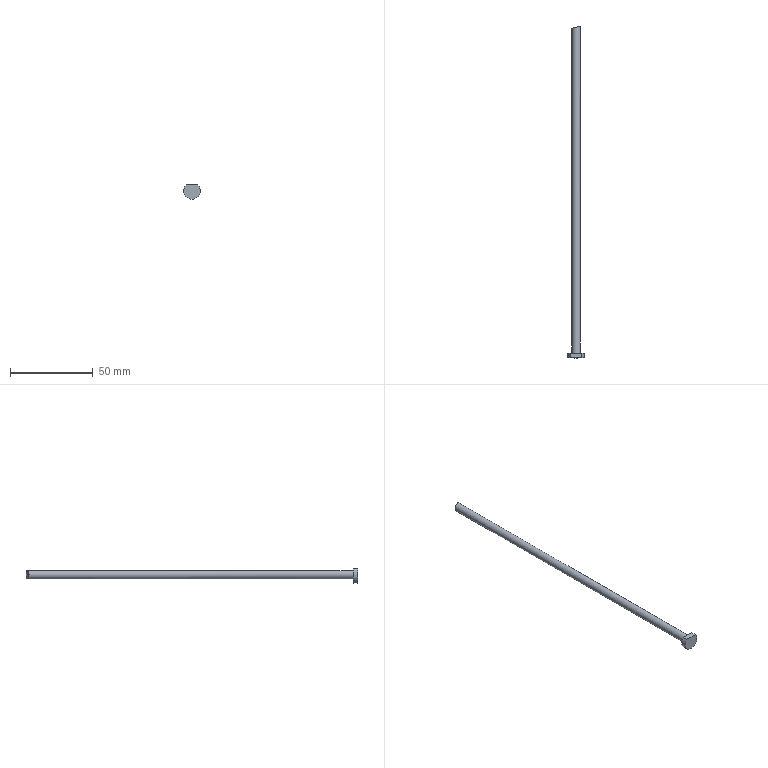Part | STEP file | EJECTION-PIN_id146_x_t | 1 solid | 8 faces | box 10 x 200.49 x 8.5 mm | volume 4074 mm3 | plane 3 | other 2 | cylinder 2 | spline 1 | commonest cylinder face diameters 5 x1 10 x1
STEP:
#1=CARTESIAN_POINT('',(22.131,-220.5,23.73));
#2=VERTEX_POINT('',#1);
#3=CARTESIAN_POINT('',(14.989,-220.5,23.73));
#4=VERTEX_POINT('',#3);
#5=CARTESIAN_POINT('',(18.56,-220.5,20.23));
#6=DIRECTION('',(0.,1.,0.));
#7=DIRECTION('',(0.,0.,1.));
#8=AXIS2_PLACEMENT_3D('',#5,#6,#7);
#9=CIRCLE('',#8,5.);
#10=EDGE_CURVE('',#2,#4,#9,.T.);
#11=ORIENTED_EDGE('',*,*,#10,.F.);
#12=CARTESIAN_POINT('',(14.989,-220.5,23.73));
#13=DIRECTION('',(1.,0.,0.));
#14=VECTOR('',#13,1.);
#15=LINE('',#12,#14);
#16=EDGE_CURVE('',#4,#2,#15,.T.);
#17=ORIENTED_EDGE('',*,*,#16,.F.);
#18=EDGE_LOOP('',(#11,#17));
#19=FACE_OUTER_BOUND('',#18,.T.);
#20=CARTESIAN_POINT('',(-30.,-220.5,27.));
#21=DIRECTION('',(0.,1.,0.));
#22=DIRECTION('',(0.,0.,1.));
#23=AXIS2_PLACEMENT_3D('',#20,#21,#22);
#24=PLANE('',#23);
#25=ADVANCED_FACE('',(#19),#24,.F.);
#26=CARTESIAN_POINT('',(16.073,-21.57,20.485));
#27=VERTEX_POINT('',#26);
#28=CARTESIAN_POINT('',(16.073,-21.57,19.976));
#29=VERTEX_POINT('',#28);
#30=CARTESIAN_POINT('',(16.073,-21.57,20.485));
#31=CARTESIAN_POINT('',(16.073,-21.595,20.485));
#32=CARTESIAN_POINT('',(16.073,-21.62,20.48));
#33=CARTESIAN_POINT('',(16.072,-21.644,20.473));
#34=CARTESIAN_POINT('',(16.071,-21.678,20.462));
#35=CARTESIAN_POINT('',(16.069,-21.711,20.446));
#36=CARTESIAN_POINT('',(16.068,-21.74,20.425));
#37=CARTESIAN_POINT('',(16.066,-21.761,20.408));
#38=CARTESIAN_POINT('',(16.065,-21.781,20.389));
#39=CARTESIAN_POINT('',(16.064,-21.797,20.366));
#40=CARTESIAN_POINT('',(16.062,-21.812,20.344));
#41=CARTESIAN_POINT('',(16.061,-21.824,20.318));
#42=CARTESIAN_POINT('',(16.061,-21.83,20.291));
#43=CARTESIAN_POINT('',(16.06,-21.835,20.271));
#44=CARTESIAN_POINT('',(16.06,-21.837,20.251));
#45=CARTESIAN_POINT('',(16.06,-21.837,20.23));
#46=CARTESIAN_POINT('',(16.06,-21.837,20.205));
#47=CARTESIAN_POINT('',(16.06,-21.834,20.18));
#48=CARTESIAN_POINT('',(16.061,-21.827,20.156));
#49=CARTESIAN_POINT('',(16.062,-21.818,20.129));
#50=CARTESIAN_POINT('',(16.063,-21.805,20.102));
#51=CARTESIAN_POINT('',(16.064,-21.787,20.08));
#52=CARTESIAN_POINT('',(16.066,-21.771,20.061));
#53=CARTESIAN_POINT('',(16.067,-21.752,20.044));
#54=CARTESIAN_POINT('',(16.068,-21.731,20.03));
#55=CARTESIAN_POINT('',(16.069,-21.707,20.013));
#56=CARTESIAN_POINT('',(16.071,-21.68,20.));
#57=CARTESIAN_POINT('',(16.072,-21.653,19.99));
#58=CARTESIAN_POINT('',(16.072,-21.626,19.981));
#59=CARTESIAN_POINT('',(16.073,-21.598,19.976));
#60=CARTESIAN_POINT('',(16.073,-21.57,19.976));
#61=B_SPLINE_CURVE_WITH_KNOTS('',3,(#30,#31,#32,#33,#34,#35,#36,#37,#38,#39,#40,#41,#42,#43,#44,#45,#46,#47,#48,#49,#50,#51,#52,#53,#54,#55,#56,#57,#58,#59,#60),.UNSPECIFIED.,.F.,.F.,(4,3,3,3,3,3,3,3,3,3,4),(0.,0.09209,0.2236,0.324,0.4253,0.5006,0.5924,0.6977,0.7892,0.8972,1.),.UNSPECIFIED.);
#62=EDGE_CURVE('',#27,#29,#61,.T.);
#63=ORIENTED_EDGE('',*,*,#62,.F.);
#64=CARTESIAN_POINT('',(21.047,-20.01,20.485));
#65=VERTEX_POINT('',#64);
#66=CARTESIAN_POINT('',(21.285,-19.924,20.485));
#67=CARTESIAN_POINT('',(20.558,-20.19,20.485));
#68=CARTESIAN_POINT('',(18.748,-20.805,20.485));
#69=CARTESIAN_POINT('',(16.921,-21.342,20.485));
#70=CARTESIAN_POINT('',(15.829,-21.636,20.485));
#71=B_SPLINE_CURVE_WITH_KNOTS('',3,(#66,#67,#68,#69,#70),.UNSPECIFIED.,.F.,.F.,(4,1,4),(0.,0.4054,1.),.UNSPECIFIED.);
#72=EDGE_CURVE('',#65,#27,#71,.T.);
#73=ORIENTED_EDGE('',*,*,#72,.F.);
#74=CARTESIAN_POINT('',(21.047,-20.01,19.976));
#75=VERTEX_POINT('',#74);
#76=CARTESIAN_POINT('',(21.047,-20.01,19.976));
#77=CARTESIAN_POINT('',(21.047,-20.035,19.976));
#78=CARTESIAN_POINT('',(21.047,-20.061,19.98));
#79=CARTESIAN_POINT('',(21.048,-20.085,19.987));
#80=CARTESIAN_POINT('',(21.049,-20.118,19.997));
#81=CARTESIAN_POINT('',(21.051,-20.15,20.013));
#82=CARTESIAN_POINT('',(21.052,-20.178,20.034));
#83=CARTESIAN_POINT('',(21.054,-20.2,20.05));
#84=CARTESIAN_POINT('',(21.055,-20.219,20.069));
#85=CARTESIAN_POINT('',(21.056,-20.235,20.091));
#86=CARTESIAN_POINT('',(21.057,-20.25,20.113));
#87=CARTESIAN_POINT('',(21.058,-20.262,20.139));
#88=CARTESIAN_POINT('',(21.059,-20.268,20.165));
#89=CARTESIAN_POINT('',(21.06,-20.274,20.186));
#90=CARTESIAN_POINT('',(21.06,-20.276,20.208));
#91=CARTESIAN_POINT('',(21.06,-20.276,20.23));
#92=CARTESIAN_POINT('',(21.06,-20.276,20.255));
#93=CARTESIAN_POINT('',(21.06,-20.273,20.28));
#94=CARTESIAN_POINT('',(21.059,-20.266,20.304));
#95=CARTESIAN_POINT('',(21.058,-20.259,20.328));
#96=CARTESIAN_POINT('',(21.057,-20.248,20.351));
#97=CARTESIAN_POINT('',(21.056,-20.234,20.371));
#98=CARTESIAN_POINT('',(21.055,-20.219,20.392));
#99=CARTESIAN_POINT('',(21.054,-20.201,20.409));
#100=CARTESIAN_POINT('',(21.052,-20.181,20.424));
#101=CARTESIAN_POINT('',(21.051,-20.153,20.445));
#102=CARTESIAN_POINT('',(21.049,-20.121,20.462));
#103=CARTESIAN_POINT('',(21.048,-20.088,20.472));
#104=CARTESIAN_POINT('',(21.047,-20.063,20.48));
#105=CARTESIAN_POINT('',(21.047,-20.037,20.485));
#106=CARTESIAN_POINT('',(21.047,-20.01,20.485));
#107=B_SPLINE_CURVE_WITH_KNOTS('',3,(#76,#77,#78,#79,#80,#81,#82,#83,#84,#85,#86,#87,#88,#89,#90,#91,#92,#93,#94,#95,#96,#97,#98,#99,#100,#101,#102,#103,#104,#105,#106),.UNSPECIFIED.,.F.,.F.,(4,3,3,3,3,3,3,3,3,3,4),(0.,0.09206,0.2207,0.3199,0.4198,0.4998,0.5915,0.6832,0.7746,0.9031,1.),.UNSPECIFIED.);
#108=EDGE_CURVE('',#75,#65,#107,.T.);
#109=ORIENTED_EDGE('',*,*,#108,.F.);
#110=CARTESIAN_POINT('',(15.829,-21.636,19.976));
#111=CARTESIAN_POINT('',(16.921,-21.342,19.976));
#112=CARTESIAN_POINT('',(18.748,-20.805,19.976));
#113=CARTESIAN_POINT('',(20.558,-20.19,19.976));
#114=CARTESIAN_POINT('',(21.285,-19.924,19.976));
#115=B_SPLINE_CURVE_WITH_KNOTS('',3,(#110,#111,#112,#113,#114),.UNSPECIFIED.,.F.,.F.,(4,1,4),(0.,0.5946,1.),.UNSPECIFIED.);
#116=EDGE_CURVE('',#29,#75,#115,.T.);
#117=ORIENTED_EDGE('',*,*,#116,.F.);
#118=EDGE_LOOP('',(#63,#73,#109,#117));
#119=FACE_OUTER_BOUND('',#118,.T.);
#120=CARTESIAN_POINT('',(15.461,-21.559,20.297));
#121=CARTESIAN_POINT('',(16.66,-21.241,20.297));
#122=CARTESIAN_POINT('',(18.673,-20.655,20.297));
#123=CARTESIAN_POINT('',(20.663,-19.975,20.297));
#124=CARTESIAN_POINT('',(21.465,-19.676,20.297));
#125=CARTESIAN_POINT('',(15.469,-21.588,20.557));
#126=CARTESIAN_POINT('',(16.668,-21.271,20.557));
#127=CARTESIAN_POINT('',(18.682,-20.684,20.557));
#128=CARTESIAN_POINT('',(20.673,-20.004,20.557));
#129=CARTESIAN_POINT('',(21.476,-19.705,20.557));
#130=CARTESIAN_POINT('',(15.555,-21.916,20.478));
#131=CARTESIAN_POINT('',(16.76,-21.597,20.478));
#132=CARTESIAN_POINT('',(18.783,-21.008,20.478));
#133=CARTESIAN_POINT('',(20.786,-20.324,20.478));
#134=CARTESIAN_POINT('',(21.594,-20.023,20.478));
#135=CARTESIAN_POINT('',(15.574,-21.986,20.23));
#136=CARTESIAN_POINT('',(16.779,-21.667,20.23));
#137=CARTESIAN_POINT('',(18.804,-21.077,20.23));
#138=CARTESIAN_POINT('',(20.81,-20.392,20.23));
#139=CARTESIAN_POINT('',(21.619,-20.09,20.23));
#140=CARTESIAN_POINT('',(15.556,-21.918,19.987));
#141=CARTESIAN_POINT('',(16.76,-21.599,19.987));
#142=CARTESIAN_POINT('',(18.783,-21.009,19.987));
#143=CARTESIAN_POINT('',(20.786,-20.325,19.987));
#144=CARTESIAN_POINT('',(21.595,-20.024,19.987));
#145=CARTESIAN_POINT('',(15.473,-21.604,19.908));
#146=CARTESIAN_POINT('',(16.673,-21.286,19.908));
#147=CARTESIAN_POINT('',(18.687,-20.699,19.908));
#148=CARTESIAN_POINT('',(20.678,-20.019,19.908));
#149=CARTESIAN_POINT('',(21.481,-19.72,19.908));
#150=CARTESIAN_POINT('',(15.462,-21.562,20.137));
#151=CARTESIAN_POINT('',(16.661,-21.245,20.137));
#152=CARTESIAN_POINT('',(18.674,-20.658,20.137));
#153=CARTESIAN_POINT('',(20.664,-19.978,20.137));
#154=CARTESIAN_POINT('',(21.466,-19.68,20.137));
#155=B_SPLINE_SURFACE_WITH_KNOTS('',3,3,((#120,#121,#122,#123,#124),(#125,#126,#127,#128,#129),(#130,#131,#132,#133,#134),(#135,#136,#137,#138,#139),(#140,#141,#142,#143,#144),(#145,#146,#147,#148,#149),(#150,#151,#152,#153,#154)),.UNSPECIFIED.,.F.,.F.,.F.,(4,1,1,1,4),(4,1,4),(0.,0.3451,0.5061,0.667,1.),(0.,0.5922,1.),.UNSPECIFIED.);
#156=ADVANCED_FACE('',(#119),#155,.F.);
#157=ORIENTED_EDGE('',*,*,#72,.T.);
#158=CARTESIAN_POINT('',(21.047,-20.01,20.485));
#159=CARTESIAN_POINT('',(21.019,-20.02,20.754));
#160=CARTESIAN_POINT('',(20.946,-20.047,21.022));
#161=CARTESIAN_POINT('',(20.835,-20.086,21.266));
#162=CARTESIAN_POINT('',(20.724,-20.126,21.51));
#163=CARTESIAN_POINT('',(20.572,-20.179,21.737));
#164=CARTESIAN_POINT('',(20.393,-20.241,21.93));
#165=CARTESIAN_POINT('',(20.208,-20.305,22.13));
#166=CARTESIAN_POINT('',(19.988,-20.38,22.299));
#167=CARTESIAN_POINT('',(19.752,-20.459,22.428));
#168=CARTESIAN_POINT('',(19.503,-20.541,22.563));
#169=CARTESIAN_POINT('',(19.229,-20.631,22.655));
#170=CARTESIAN_POINT('',(18.951,-20.719,22.699));
#171=CARTESIAN_POINT('',(18.663,-20.811,22.745));
#172=CARTESIAN_POINT('',(18.363,-20.904,22.739));
#173=CARTESIAN_POINT('',(18.076,-20.992,22.683));
#174=CARTESIAN_POINT('',(17.788,-21.08,22.626));
#175=CARTESIAN_POINT('',(17.505,-21.164,22.516));
#176=CARTESIAN_POINT('',(17.251,-21.238,22.36));
#177=CARTESIAN_POINT('',(17.004,-21.31,22.208));
#178=CARTESIAN_POINT('',(16.779,-21.374,22.009));
#179=CARTESIAN_POINT('',(16.597,-21.425,21.778));
#180=CARTESIAN_POINT('',(16.422,-21.474,21.556));
#181=CARTESIAN_POINT('',(16.282,-21.513,21.298));
#182=CARTESIAN_POINT('',(16.191,-21.538,21.027));
#183=CARTESIAN_POINT('',(16.132,-21.554,20.852));
#184=CARTESIAN_POINT('',(16.092,-21.565,20.669));
#185=CARTESIAN_POINT('',(16.073,-21.57,20.485));
#186=B_SPLINE_CURVE_WITH_KNOTS('',3,(#158,#159,#160,#161,#162,#163,#164,#165,#166,#167,#168,#169,#170,#171,#172,#173,#174,#175,#176,#177,#178,#179,#180,#181,#182,#183,#184,#185),.UNSPECIFIED.,.F.,.F.,(4,3,3,3,3,3,3,3,3,4),(0.,0.1085,0.2168,0.3287,0.4468,0.569,0.6918,0.8115,0.9264,1.),.UNSPECIFIED.);
#187=EDGE_CURVE('',#65,#27,#186,.T.);
#188=ORIENTED_EDGE('',*,*,#187,.F.);
#189=EDGE_LOOP('',(#157,#188));
#190=FACE_OUTER_BOUND('',#189,.T.);
#191=CARTESIAN_POINT('',(15.829,-21.636,25.066));
#192=CARTESIAN_POINT('',(16.921,-21.342,25.066));
#193=CARTESIAN_POINT('',(18.748,-20.805,25.066));
#194=CARTESIAN_POINT('',(20.558,-20.19,25.066));
#195=CARTESIAN_POINT('',(21.285,-19.924,25.066));
#196=(BOUNDED_CURVE()B_SPLINE_CURVE(3,(#191,#192,#193,#194,#195),.UNSPECIFIED.,.F.,.F.)B_SPLINE_CURVE_WITH_KNOTS((4,1,4),(0.,0.5946,1.),.UNSPECIFIED.)CURVE()GEOMETRIC_REPRESENTATION_ITEM()RATIONAL_B_SPLINE_CURVE((1.,1.,1.,1.,1.))REPRESENTATION_ITEM(''));
#197=DIRECTION('',(0.,0.,-1.));
#198=VECTOR('',#197,1.);
#199=SURFACE_OF_LINEAR_EXTRUSION('',#196,#198);
#200=ADVANCED_FACE('',(#190),#199,.T.);
#201=CARTESIAN_POINT('',(14.989,-217.5,23.73));
#202=VERTEX_POINT('',#201);
#203=CARTESIAN_POINT('',(14.989,-220.5,23.73));
#204=DIRECTION('',(0.,1.,0.));
#205=VECTOR('',#204,1.);
#206=LINE('',#203,#205);
#207=EDGE_CURVE('',#4,#202,#206,.T.);
#208=ORIENTED_EDGE('',*,*,#207,.F.);
#209=ORIENTED_EDGE('',*,*,#16,.T.);
#210=CARTESIAN_POINT('',(22.131,-217.5,23.73));
#211=VERTEX_POINT('',#210);
#212=CARTESIAN_POINT('',(22.131,-220.5,23.73));
#213=DIRECTION('',(0.,-1.,0.));
#214=VECTOR('',#213,1.);
#215=LINE('',#212,#214);
#216=EDGE_CURVE('',#211,#2,#215,.T.);
#217=ORIENTED_EDGE('',*,*,#216,.F.);
#218=CARTESIAN_POINT('',(130.,-217.5,23.73));
#219=DIRECTION('',(1.,0.,0.));
#220=VECTOR('',#219,1.);
#221=LINE('',#218,#220);
#222=EDGE_CURVE('',#202,#211,#221,.T.);
#223=ORIENTED_EDGE('',*,*,#222,.F.);
#224=EDGE_LOOP('',(#208,#209,#217,#223));
#225=FACE_OUTER_BOUND('',#224,.T.);
#226=CARTESIAN_POINT('',(14.989,-220.5,23.73));
#227=DIRECTION('',(0.,0.,1.));
#228=DIRECTION('',(1.,0.,0.));
#229=AXIS2_PLACEMENT_3D('',#226,#227,#228);
#230=PLANE('',#229);
#231=ADVANCED_FACE('',(#225),#230,.T.);
#232=ORIENTED_EDGE('',*,*,#216,.T.);
#233=ORIENTED_EDGE('',*,*,#10,.T.);
#234=ORIENTED_EDGE('',*,*,#207,.T.);
#235=CARTESIAN_POINT('',(18.56,-217.5,20.23));
#236=DIRECTION('',(0.,1.,0.));
#237=DIRECTION('',(0.,0.,1.));
#238=AXIS2_PLACEMENT_3D('',#235,#236,#237);
#239=CIRCLE('',#238,5.);
#240=EDGE_CURVE('',#211,#202,#239,.T.);
#241=ORIENTED_EDGE('',*,*,#240,.F.);
#242=EDGE_LOOP('',(#232,#233,#234,#241));
#243=FACE_OUTER_BOUND('',#242,.T.);
#244=CARTESIAN_POINT('',(18.56,-220.5,20.23));
#245=DIRECTION('',(0.,1.,0.));
#246=DIRECTION('',(0.,0.,1.));
#247=AXIS2_PLACEMENT_3D('',#244,#245,#246);
#248=CYLINDRICAL_SURFACE('',#247,5.);
#249=ADVANCED_FACE('',(#243),#248,.T.);
#250=ORIENTED_EDGE('',*,*,#116,.T.);
#251=CARTESIAN_POINT('',(16.073,-21.57,19.976));
#252=CARTESIAN_POINT('',(16.101,-21.562,19.704));
#253=CARTESIAN_POINT('',(16.175,-21.542,19.433));
#254=CARTESIAN_POINT('',(16.289,-21.511,19.185));
#255=CARTESIAN_POINT('',(16.402,-21.479,18.939));
#256=CARTESIAN_POINT('',(16.558,-21.436,18.709));
#257=CARTESIAN_POINT('',(16.742,-21.384,18.513));
#258=CARTESIAN_POINT('',(16.93,-21.331,18.315));
#259=CARTESIAN_POINT('',(17.152,-21.267,18.146));
#260=CARTESIAN_POINT('',(17.391,-21.197,18.02));
#261=CARTESIAN_POINT('',(17.638,-21.124,17.89));
#262=CARTESIAN_POINT('',(17.909,-21.043,17.801));
#263=CARTESIAN_POINT('',(18.182,-20.96,17.759));
#264=CARTESIAN_POINT('',(18.465,-20.873,17.715));
#265=CARTESIAN_POINT('',(18.759,-20.781,17.722));
#266=CARTESIAN_POINT('',(19.04,-20.691,17.776));
#267=CARTESIAN_POINT('',(19.327,-20.599,17.833));
#268=CARTESIAN_POINT('',(19.608,-20.507,17.941));
#269=CARTESIAN_POINT('',(19.86,-20.422,18.095));
#270=CARTESIAN_POINT('',(20.111,-20.339,18.247));
#271=CARTESIAN_POINT('',(20.339,-20.26,18.448));
#272=CARTESIAN_POINT('',(20.523,-20.196,18.682));
#273=CARTESIAN_POINT('',(20.701,-20.134,18.907));
#274=CARTESIAN_POINT('',(20.843,-20.084,19.17));
#275=CARTESIAN_POINT('',(20.934,-20.051,19.446));
#276=CARTESIAN_POINT('',(20.99,-20.031,19.617));
#277=CARTESIAN_POINT('',(21.029,-20.017,19.796));
#278=CARTESIAN_POINT('',(21.047,-20.01,19.976));
#279=B_SPLINE_CURVE_WITH_KNOTS('',3,(#251,#252,#253,#254,#255,#256,#257,#258,#259,#260,#261,#262,#263,#264,#265,#266,#267,#268,#269,#270,#271,#272,#273,#274,#275,#276,#277,#278),.UNSPECIFIED.,.F.,.F.,(4,3,3,3,3,3,3,3,3,4),(0.,0.1095,0.2189,0.3303,0.4458,0.5657,0.6886,0.8107,0.9282,1.),.UNSPECIFIED.);
#280=EDGE_CURVE('',#29,#75,#279,.T.);
#281=ORIENTED_EDGE('',*,*,#280,.F.);
#282=EDGE_LOOP('',(#250,#281));
#283=FACE_OUTER_BOUND('',#282,.T.);
#284=CARTESIAN_POINT('',(15.829,-21.636,19.976));
#285=CARTESIAN_POINT('',(16.921,-21.342,19.976));
#286=CARTESIAN_POINT('',(18.748,-20.805,19.976));
#287=CARTESIAN_POINT('',(20.558,-20.19,19.976));
#288=CARTESIAN_POINT('',(21.285,-19.924,19.976));
#289=(BOUNDED_CURVE()B_SPLINE_CURVE(3,(#284,#285,#286,#287,#288),.UNSPECIFIED.,.F.,.F.)B_SPLINE_CURVE_WITH_KNOTS((4,1,4),(0.,0.5946,1.),.UNSPECIFIED.)CURVE()GEOMETRIC_REPRESENTATION_ITEM()RATIONAL_B_SPLINE_CURVE((1.,1.,1.,1.,1.))REPRESENTATION_ITEM(''));
#290=DIRECTION('',(0.,0.,-1.));
#291=VECTOR('',#290,1.);
#292=SURFACE_OF_LINEAR_EXTRUSION('',#289,#291);
#293=ADVANCED_FACE('',(#283),#292,.T.);
#294=CARTESIAN_POINT('',(18.56,-217.5,22.73));
#295=VERTEX_POINT('',#294);
#296=CARTESIAN_POINT('',(18.56,-217.5,20.23));
#297=DIRECTION('',(0.,1.,0.));
#298=DIRECTION('',(0.,0.,1.));
#299=AXIS2_PLACEMENT_3D('',#296,#297,#298);
#300=CIRCLE('',#299,2.5);
#301=EDGE_CURVE('',#295,#295,#300,.T.);
#302=ORIENTED_EDGE('',*,*,#301,.F.);
#303=EDGE_LOOP('',(#302));
#304=FACE_BOUND('',#303,.T.);
#305=ORIENTED_EDGE('',*,*,#222,.T.);
#306=ORIENTED_EDGE('',*,*,#240,.T.);
#307=EDGE_LOOP('',(#305,#306));
#308=FACE_BOUND('',#307,.T.);
#309=CARTESIAN_POINT('',(130.,-217.5,-52.5));
#310=DIRECTION('',(0.,1.,0.));
#311=DIRECTION('',(0.,0.,1.));
#312=AXIS2_PLACEMENT_3D('',#309,#310,#311);
#313=PLANE('',#312);
#314=ADVANCED_FACE('',(#304,#308),#313,.T.);
#315=ORIENTED_EDGE('',*,*,#187,.T.);
#316=ORIENTED_EDGE('',*,*,#62,.T.);
#317=ORIENTED_EDGE('',*,*,#280,.T.);
#318=ORIENTED_EDGE('',*,*,#108,.T.);
#319=EDGE_LOOP('',(#315,#316,#317,#318));
#320=FACE_BOUND('',#319,.T.);
#321=ORIENTED_EDGE('',*,*,#301,.T.);
#322=EDGE_LOOP('',(#321));
#323=FACE_BOUND('',#322,.T.);
#324=CARTESIAN_POINT('',(18.56,0.,20.23));
#325=DIRECTION('',(0.,1.,0.));
#326=DIRECTION('',(0.,0.,1.));
#327=AXIS2_PLACEMENT_3D('',#324,#325,#326);
#328=CYLINDRICAL_SURFACE('',#327,2.5);
#329=ADVANCED_FACE('',(#320,#323),#328,.T.);
#330=CLOSED_SHELL('',(#25,#156,#200,#231,#249,#293,#314,#329));
#331=MANIFOLD_SOLID_BREP('',#330);
#332=(LENGTH_UNIT()NAMED_UNIT(*)SI_UNIT(.MILLI.,.METRE.));
#333=UNCERTAINTY_MEASURE_WITH_UNIT(LENGTH_MEASURE(0.0508),#332,'','');
#334=(NAMED_UNIT(*)PLANE_ANGLE_UNIT()SI_UNIT($,.RADIAN.));
#335=PLANE_ANGLE_MEASURE_WITH_UNIT(PLANE_ANGLE_MEASURE(0.01745),#334);
#336=DIMENSIONAL_EXPONENTS(0.,0.,0.,0.,0.,0.,0.);
#337=(CONVERSION_BASED_UNIT('DEGREE',#335)NAMED_UNIT(#336)PLANE_ANGLE_UNIT());
#338=(NAMED_UNIT(*)SI_UNIT($,.STERADIAN.)SOLID_ANGLE_UNIT());
#339=(GEOMETRIC_REPRESENTATION_CONTEXT(3)GLOBAL_UNCERTAINTY_ASSIGNED_CONTEXT((#333))GLOBAL_UNIT_ASSIGNED_CONTEXT((#332,#337,#338))REPRESENTATION_CONTEXT('',''));
#340=ADVANCED_BREP_SHAPE_REPRESENTATION('',(#331),#339);